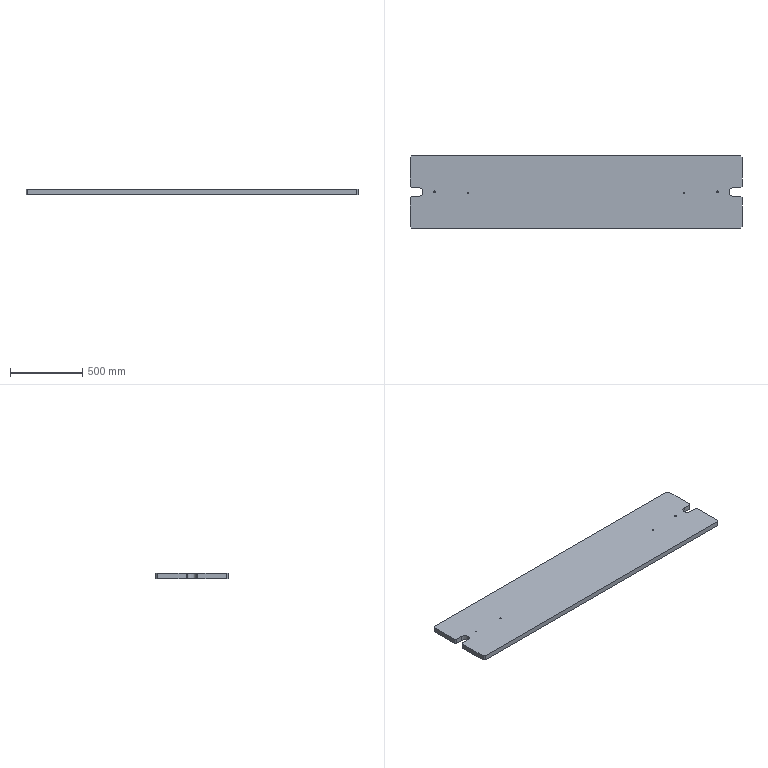Part | SolidWorks | features ICE 3, Cut 2, HoleWzd 2, Chamfer 1, Extrusion 1 | 1 solid | 106 faces | box 2300 x 500 x 35 mm | volume 39674536 mm3 | cylinder 56 | plane 34 | cone 16 | commonest cylinder face diameters 6.8 x16 80 x15 6.6 x8 11 x8 5 x6 60 x3